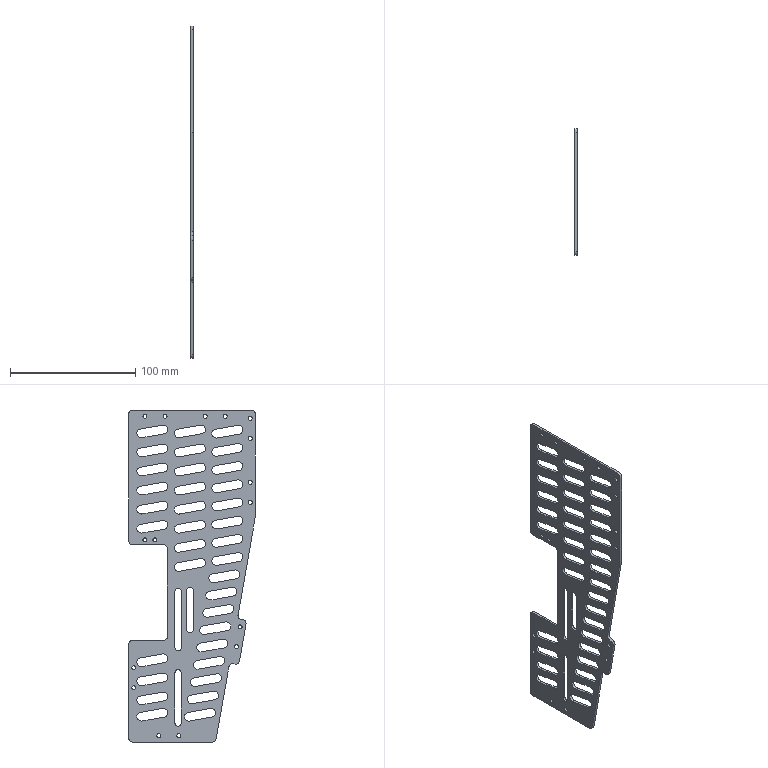Part | SolidWorks | features ICE 9, Fillet 3, Extrusion 1 | 1 solid | 251 faces | box 2 x 101 x 264.6 mm | volume 30475 mm3 | cylinder 160 | plane 91 | commonest cylinder face diameters 7 x105 3.2 x32 6 x17 5 x6